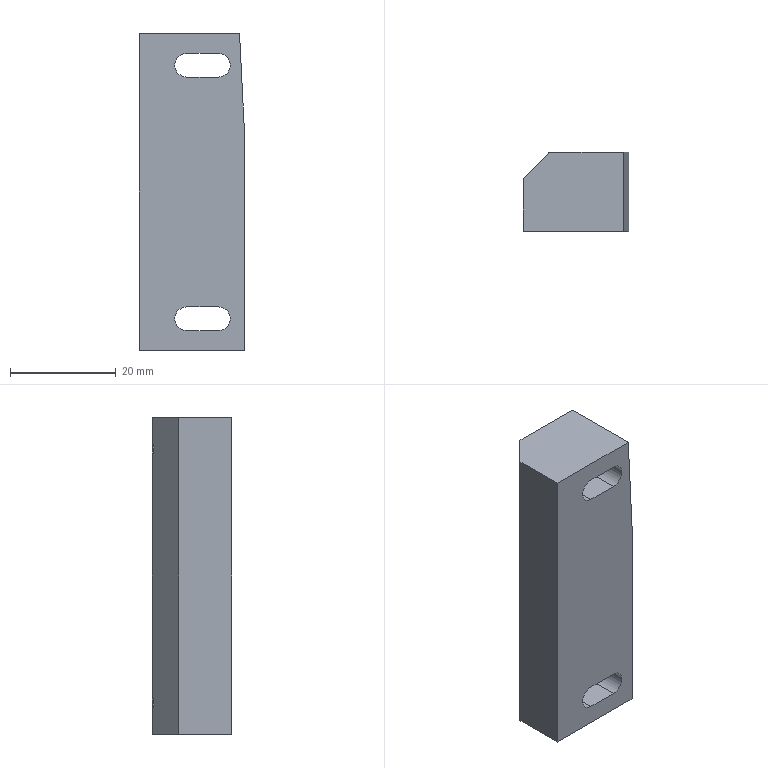Part | SolidWorks | features Cut 3, Chamfer 1, Extrusion 1, MirrorPattern 1 | 1 solid | 26 faces | box 20 x 15 x 60 mm | volume 15035 mm3 | plane 18 | cylinder 8 | commonest cylinder face diameters 4.5 x4 8.5 x4
STEP:
#1=CARTESIAN_POINT('',(-5.,15.,-22.564));
#2=VERTEX_POINT('',#1);
#3=CARTESIAN_POINT('',(-5.,15.,22.564));
#4=VERTEX_POINT('',#3);
#5=CARTESIAN_POINT('',(-5.,15.,30.));
#6=DIRECTION('',(0.,0.,1.));
#7=VECTOR('',#6,1000.);
#8=LINE('',#5,#7);
#9=EDGE_CURVE('',#2,#4,#8,.T.);
#10=ORIENTED_EDGE('',*,*,#9,.T.);
#11=CARTESIAN_POINT('',(-1.,15.,19.75));
#12=VERTEX_POINT('',#11);
#13=CARTESIAN_POINT('',(-1.,15.,24.));
#14=DIRECTION('',(0.,-1.,0.));
#15=DIRECTION('',(0.,0.,-1.));
#16=AXIS2_PLACEMENT_3D('',#13,#14,#15);
#17=CIRCLE('',#16,4.25);
#18=EDGE_CURVE('',#4,#12,#17,.T.);
#19=ORIENTED_EDGE('',*,*,#18,.T.);
#20=CARTESIAN_POINT('',(5.,15.,19.75));
#21=VERTEX_POINT('',#20);
#22=CARTESIAN_POINT('',(-1.,15.,19.75));
#23=DIRECTION('',(1.,0.,0.));
#24=VECTOR('',#23,1000.);
#25=LINE('',#22,#24);
#26=EDGE_CURVE('',#12,#21,#25,.T.);
#27=ORIENTED_EDGE('',*,*,#26,.T.);
#28=CARTESIAN_POINT('',(5.,15.,28.25));
#29=VERTEX_POINT('',#28);
#30=CARTESIAN_POINT('',(5.,15.,24.));
#31=DIRECTION('',(0.,-1.,0.));
#32=DIRECTION('',(0.,0.,-1.));
#33=AXIS2_PLACEMENT_3D('',#30,#31,#32);
#34=CIRCLE('',#33,4.25);
#35=EDGE_CURVE('',#21,#29,#34,.T.);
#36=ORIENTED_EDGE('',*,*,#35,.T.);
#37=CARTESIAN_POINT('',(-1.,15.,28.25));
#38=VERTEX_POINT('',#37);
#39=CARTESIAN_POINT('',(5.,15.,28.25));
#40=DIRECTION('',(-1.,0.,0.));
#41=VECTOR('',#40,1000.);
#42=LINE('',#39,#41);
#43=EDGE_CURVE('',#29,#38,#42,.T.);
#44=ORIENTED_EDGE('',*,*,#43,.T.);
#45=CARTESIAN_POINT('',(-5.,15.,25.436));
#46=VERTEX_POINT('',#45);
#47=CARTESIAN_POINT('',(-1.,15.,24.));
#48=DIRECTION('',(0.,-1.,0.));
#49=DIRECTION('',(0.,0.,-1.));
#50=AXIS2_PLACEMENT_3D('',#47,#48,#49);
#51=CIRCLE('',#50,4.25);
#52=EDGE_CURVE('',#38,#46,#51,.T.);
#53=ORIENTED_EDGE('',*,*,#52,.T.);
#54=CARTESIAN_POINT('',(-5.,15.,30.));
#55=VERTEX_POINT('',#54);
#56=CARTESIAN_POINT('',(-5.,15.,30.));
#57=DIRECTION('',(0.,0.,1.));
#58=VECTOR('',#57,1000.);
#59=LINE('',#56,#58);
#60=EDGE_CURVE('',#46,#55,#59,.T.);
#61=ORIENTED_EDGE('',*,*,#60,.T.);
#62=CARTESIAN_POINT('',(9.,15.,30.));
#63=VERTEX_POINT('',#62);
#64=CARTESIAN_POINT('',(-10.,15.,30.));
#65=DIRECTION('',(1.,0.,0.));
#66=VECTOR('',#65,1000.);
#67=LINE('',#64,#66);
#68=EDGE_CURVE('',#55,#63,#67,.T.);
#69=ORIENTED_EDGE('',*,*,#68,.T.);
#70=CARTESIAN_POINT('',(10.,15.,10.));
#71=VERTEX_POINT('',#70);
#72=CARTESIAN_POINT('',(9.,15.,30.));
#73=DIRECTION('',(-0.04994,0.,0.9988));
#74=VECTOR('',#73,1000.);
#75=LINE('',#72,#74);
#76=EDGE_CURVE('',#71,#63,#75,.T.);
#77=ORIENTED_EDGE('',*,*,#76,.F.);
#78=CARTESIAN_POINT('',(10.,15.,-30.));
#79=VERTEX_POINT('',#78);
#80=CARTESIAN_POINT('',(10.,15.,-30.));
#81=DIRECTION('',(0.,0.,-1.));
#82=VECTOR('',#81,1000.);
#83=LINE('',#80,#82);
#84=EDGE_CURVE('',#71,#79,#83,.T.);
#85=ORIENTED_EDGE('',*,*,#84,.T.);
#86=CARTESIAN_POINT('',(-5.,15.,-30.));
#87=VERTEX_POINT('',#86);
#88=CARTESIAN_POINT('',(-10.,15.,-30.));
#89=DIRECTION('',(-1.,0.,0.));
#90=VECTOR('',#89,1000.);
#91=LINE('',#88,#90);
#92=EDGE_CURVE('',#79,#87,#91,.T.);
#93=ORIENTED_EDGE('',*,*,#92,.T.);
#94=CARTESIAN_POINT('',(-5.,15.,-25.436));
#95=VERTEX_POINT('',#94);
#96=CARTESIAN_POINT('',(-5.,15.,30.));
#97=DIRECTION('',(0.,0.,1.));
#98=VECTOR('',#97,1000.);
#99=LINE('',#96,#98);
#100=EDGE_CURVE('',#87,#95,#99,.T.);
#101=ORIENTED_EDGE('',*,*,#100,.T.);
#102=CARTESIAN_POINT('',(-1.,15.,-28.25));
#103=VERTEX_POINT('',#102);
#104=CARTESIAN_POINT('',(-1.,15.,-24.));
#105=DIRECTION('',(0.,1.,0.));
#106=DIRECTION('',(0.,0.,1.));
#107=AXIS2_PLACEMENT_3D('',#104,#105,#106);
#108=CIRCLE('',#107,4.25);
#109=EDGE_CURVE('',#103,#95,#108,.T.);
#110=ORIENTED_EDGE('',*,*,#109,.F.);
#111=CARTESIAN_POINT('',(5.,15.,-28.25));
#112=VERTEX_POINT('',#111);
#113=CARTESIAN_POINT('',(5.,15.,-28.25));
#114=DIRECTION('',(-1.,0.,0.));
#115=VECTOR('',#114,1000.);
#116=LINE('',#113,#115);
#117=EDGE_CURVE('',#112,#103,#116,.T.);
#118=ORIENTED_EDGE('',*,*,#117,.F.);
#119=CARTESIAN_POINT('',(5.,15.,-19.75));
#120=VERTEX_POINT('',#119);
#121=CARTESIAN_POINT('',(5.,15.,-24.));
#122=DIRECTION('',(0.,1.,0.));
#123=DIRECTION('',(0.,0.,1.));
#124=AXIS2_PLACEMENT_3D('',#121,#122,#123);
#125=CIRCLE('',#124,4.25);
#126=EDGE_CURVE('',#120,#112,#125,.T.);
#127=ORIENTED_EDGE('',*,*,#126,.F.);
#128=CARTESIAN_POINT('',(-1.,15.,-19.75));
#129=VERTEX_POINT('',#128);
#130=CARTESIAN_POINT('',(-1.,15.,-19.75));
#131=DIRECTION('',(1.,0.,0.));
#132=VECTOR('',#131,1000.);
#133=LINE('',#130,#132);
#134=EDGE_CURVE('',#129,#120,#133,.T.);
#135=ORIENTED_EDGE('',*,*,#134,.F.);
#136=CARTESIAN_POINT('',(-1.,15.,-24.));
#137=DIRECTION('',(0.,1.,0.));
#138=DIRECTION('',(0.,0.,1.));
#139=AXIS2_PLACEMENT_3D('',#136,#137,#138);
#140=CIRCLE('',#139,4.25);
#141=EDGE_CURVE('',#2,#129,#140,.T.);
#142=ORIENTED_EDGE('',*,*,#141,.F.);
#143=EDGE_LOOP('',(#10,#19,#27,#36,#44,#53,#61,#69,#77,#85,#93,#101,#110,#118,#127,#135,#142));
#144=FACE_OUTER_BOUND('',#143,.T.);
#145=CARTESIAN_POINT('',(0.,15.,0.));
#146=DIRECTION('',(0.,1.,0.));
#147=DIRECTION('',(0.,0.,1.));
#148=AXIS2_PLACEMENT_3D('',#145,#146,#147);
#149=PLANE('',#148);
#150=ADVANCED_FACE('',(#144),#149,.T.);
#151=ORIENTED_EDGE('',*,*,#60,.F.);
#152=CARTESIAN_POINT('',(-5.,15.,25.436));
#153=CARTESIAN_POINT('',(-5.337,14.663,24.498));
#154=CARTESIAN_POINT('',(-5.337,14.663,23.502));
#155=CARTESIAN_POINT('',(-5.,15.,22.564));
#156=(BOUNDED_CURVE()B_SPLINE_CURVE(3,(#152,#153,#154,#155),.UNSPECIFIED.,.F.,.F.)B_SPLINE_CURVE_WITH_KNOTS((4,4),(2.797,3.486),.UNSPECIFIED.)CURVE()GEOMETRIC_REPRESENTATION_ITEM()RATIONAL_B_SPLINE_CURVE((1.,0.9608,0.9608,1.))REPRESENTATION_ITEM(''));
#157=EDGE_CURVE('',#46,#4,#156,.T.);
#158=ORIENTED_EDGE('',*,*,#157,.T.);
#159=ORIENTED_EDGE('',*,*,#9,.F.);
#160=CARTESIAN_POINT('',(-5.,15.,-25.436));
#161=CARTESIAN_POINT('',(-5.337,14.663,-24.498));
#162=CARTESIAN_POINT('',(-5.337,14.663,-23.502));
#163=CARTESIAN_POINT('',(-5.,15.,-22.564));
#164=(BOUNDED_CURVE()B_SPLINE_CURVE(3,(#160,#161,#162,#163),.UNSPECIFIED.,.F.,.F.)B_SPLINE_CURVE_WITH_KNOTS((4,4),(2.797,3.486),.UNSPECIFIED.)CURVE()GEOMETRIC_REPRESENTATION_ITEM()RATIONAL_B_SPLINE_CURVE((1.,0.9608,0.9608,1.))REPRESENTATION_ITEM(''));
#165=EDGE_CURVE('',#95,#2,#164,.T.);
#166=ORIENTED_EDGE('',*,*,#165,.F.);
#167=ORIENTED_EDGE('',*,*,#100,.F.);
#168=CARTESIAN_POINT('',(-10.,10.,-30.));
#169=VERTEX_POINT('',#168);
#170=CARTESIAN_POINT('',(-5.,15.,-30.));
#171=DIRECTION('',(0.7071,0.7071,0.));
#172=VECTOR('',#171,1000.);
#173=LINE('',#170,#172);
#174=EDGE_CURVE('',#169,#87,#173,.T.);
#175=ORIENTED_EDGE('',*,*,#174,.F.);
#176=CARTESIAN_POINT('',(-10.,10.,30.));
#177=VERTEX_POINT('',#176);
#178=CARTESIAN_POINT('',(-10.,10.,-30.));
#179=DIRECTION('',(0.,0.,-1.));
#180=VECTOR('',#179,1000.);
#181=LINE('',#178,#180);
#182=EDGE_CURVE('',#177,#169,#181,.T.);
#183=ORIENTED_EDGE('',*,*,#182,.F.);
#184=CARTESIAN_POINT('',(-5.,15.,30.));
#185=DIRECTION('',(-0.7071,-0.7071,0.));
#186=VECTOR('',#185,1000.);
#187=LINE('',#184,#186);
#188=EDGE_CURVE('',#55,#177,#187,.T.);
#189=ORIENTED_EDGE('',*,*,#188,.F.);
#190=EDGE_LOOP('',(#151,#158,#159,#166,#167,#175,#183,#189));
#191=FACE_OUTER_BOUND('',#190,.T.);
#192=CARTESIAN_POINT('',(-5.,15.,0.));
#193=DIRECTION('',(-0.7071,0.7071,0.));
#194=DIRECTION('',(0.,0.,-1.));
#195=AXIS2_PLACEMENT_3D('',#192,#193,#194);
#196=PLANE('',#195);
#197=ADVANCED_FACE('',(#191),#196,.T.);
#198=CARTESIAN_POINT('',(5.,0.,26.25));
#199=VERTEX_POINT('',#198);
#200=CARTESIAN_POINT('',(5.,9.,26.25));
#201=VERTEX_POINT('',#200);
#202=CARTESIAN_POINT('',(5.,0.,26.25));
#203=DIRECTION('',(0.,1.,0.));
#204=VECTOR('',#203,1000.);
#205=LINE('',#202,#204);
#206=EDGE_CURVE('',#199,#201,#205,.T.);
#207=ORIENTED_EDGE('',*,*,#206,.T.);
#208=CARTESIAN_POINT('',(5.,9.,21.75));
#209=VERTEX_POINT('',#208);
#210=CARTESIAN_POINT('',(5.,9.,24.));
#211=DIRECTION('',(0.,1.,0.));
#212=DIRECTION('',(0.,0.,1.));
#213=AXIS2_PLACEMENT_3D('',#210,#211,#212);
#214=CIRCLE('',#213,2.25);
#215=EDGE_CURVE('',#201,#209,#214,.T.);
#216=ORIENTED_EDGE('',*,*,#215,.T.);
#217=CARTESIAN_POINT('',(5.,0.,21.75));
#218=VERTEX_POINT('',#217);
#219=CARTESIAN_POINT('',(5.,0.,21.75));
#220=DIRECTION('',(0.,1.,0.));
#221=VECTOR('',#220,1000.);
#222=LINE('',#219,#221);
#223=EDGE_CURVE('',#218,#209,#222,.T.);
#224=ORIENTED_EDGE('',*,*,#223,.F.);
#225=CARTESIAN_POINT('',(5.,0.,24.));
#226=DIRECTION('',(0.,-1.,0.));
#227=DIRECTION('',(0.,0.,-1.));
#228=AXIS2_PLACEMENT_3D('',#225,#226,#227);
#229=CIRCLE('',#228,2.25);
#230=EDGE_CURVE('',#218,#199,#229,.T.);
#231=ORIENTED_EDGE('',*,*,#230,.T.);
#232=EDGE_LOOP('',(#207,#216,#224,#231));
#233=FACE_OUTER_BOUND('',#232,.T.);
#234=CARTESIAN_POINT('',(5.,0.,24.));
#235=DIRECTION('',(0.,1.,0.));
#236=DIRECTION('',(0.,0.,1.));
#237=AXIS2_PLACEMENT_3D('',#234,#235,#236);
#238=CYLINDRICAL_SURFACE('',#237,2.25);
#239=ADVANCED_FACE('',(#233),#238,.F.);
#240=CARTESIAN_POINT('',(-1.,0.,26.25));
#241=VERTEX_POINT('',#240);
#242=CARTESIAN_POINT('',(-1.,9.,26.25));
#243=VERTEX_POINT('',#242);
#244=CARTESIAN_POINT('',(-1.,0.,26.25));
#245=DIRECTION('',(0.,1.,0.));
#246=VECTOR('',#245,1000.);
#247=LINE('',#244,#246);
#248=EDGE_CURVE('',#241,#243,#247,.T.);
#249=ORIENTED_EDGE('',*,*,#248,.T.);
#250=CARTESIAN_POINT('',(5.,9.,26.25));
#251=DIRECTION('',(1.,0.,0.));
#252=VECTOR('',#251,1000.);
#253=LINE('',#250,#252);
#254=EDGE_CURVE('',#243,#201,#253,.T.);
#255=ORIENTED_EDGE('',*,*,#254,.T.);
#256=ORIENTED_EDGE('',*,*,#206,.F.);
#257=CARTESIAN_POINT('',(5.,0.,26.25));
#258=DIRECTION('',(-1.,0.,0.));
#259=VECTOR('',#258,1000.);
#260=LINE('',#257,#259);
#261=EDGE_CURVE('',#199,#241,#260,.T.);
#262=ORIENTED_EDGE('',*,*,#261,.T.);
#263=EDGE_LOOP('',(#249,#255,#256,#262));
#264=FACE_OUTER_BOUND('',#263,.T.);
#265=CARTESIAN_POINT('',(5.,0.,26.25));
#266=DIRECTION('',(0.,0.,-1.));
#267=DIRECTION('',(-1.,0.,0.));
#268=AXIS2_PLACEMENT_3D('',#265,#266,#267);
#269=PLANE('',#268);
#270=ADVANCED_FACE('',(#264),#269,.T.);
#271=CARTESIAN_POINT('',(-1.,0.,21.75));
#272=VERTEX_POINT('',#271);
#273=CARTESIAN_POINT('',(-1.,9.,21.75));
#274=VERTEX_POINT('',#273);
#275=CARTESIAN_POINT('',(-1.,0.,21.75));
#276=DIRECTION('',(0.,1.,0.));
#277=VECTOR('',#276,1000.);
#278=LINE('',#275,#277);
#279=EDGE_CURVE('',#272,#274,#278,.T.);
#280=ORIENTED_EDGE('',*,*,#279,.T.);
#281=CARTESIAN_POINT('',(-1.,9.,24.));
#282=DIRECTION('',(0.,1.,0.));
#283=DIRECTION('',(0.,0.,1.));
#284=AXIS2_PLACEMENT_3D('',#281,#282,#283);
#285=CIRCLE('',#284,2.25);
#286=EDGE_CURVE('',#274,#243,#285,.T.);
#287=ORIENTED_EDGE('',*,*,#286,.T.);
#288=ORIENTED_EDGE('',*,*,#248,.F.);
#289=CARTESIAN_POINT('',(-1.,0.,24.));
#290=DIRECTION('',(0.,-1.,0.));
#291=DIRECTION('',(0.,0.,-1.));
#292=AXIS2_PLACEMENT_3D('',#289,#290,#291);
#293=CIRCLE('',#292,2.25);
#294=EDGE_CURVE('',#241,#272,#293,.T.);
#295=ORIENTED_EDGE('',*,*,#294,.T.);
#296=EDGE_LOOP('',(#280,#287,#288,#295));
#297=FACE_OUTER_BOUND('',#296,.T.);
#298=CARTESIAN_POINT('',(-1.,0.,24.));
#299=DIRECTION('',(0.,1.,0.));
#300=DIRECTION('',(0.,0.,1.));
#301=AXIS2_PLACEMENT_3D('',#298,#299,#300);
#302=CYLINDRICAL_SURFACE('',#301,2.25);
#303=ADVANCED_FACE('',(#297),#302,.F.);
#304=ORIENTED_EDGE('',*,*,#223,.T.);
#305=CARTESIAN_POINT('',(5.,9.,21.75));
#306=DIRECTION('',(-1.,0.,0.));
#307=VECTOR('',#306,1000.);
#308=LINE('',#305,#307);
#309=EDGE_CURVE('',#209,#274,#308,.T.);
#310=ORIENTED_EDGE('',*,*,#309,.T.);
#311=ORIENTED_EDGE('',*,*,#279,.F.);
#312=CARTESIAN_POINT('',(5.,0.,21.75));
#313=DIRECTION('',(1.,0.,0.));
#314=VECTOR('',#313,1000.);
#315=LINE('',#312,#314);
#316=EDGE_CURVE('',#272,#218,#315,.T.);
#317=ORIENTED_EDGE('',*,*,#316,.T.);
#318=EDGE_LOOP('',(#304,#310,#311,#317));
#319=FACE_OUTER_BOUND('',#318,.T.);
#320=CARTESIAN_POINT('',(5.,0.,21.75));
#321=DIRECTION('',(0.,0.,1.));
#322=DIRECTION('',(1.,0.,0.));
#323=AXIS2_PLACEMENT_3D('',#320,#321,#322);
#324=PLANE('',#323);
#325=ADVANCED_FACE('',(#319),#324,.T.);
#326=CARTESIAN_POINT('',(10.,0.,10.));
#327=VERTEX_POINT('',#326);
#328=CARTESIAN_POINT('',(10.,0.,-30.));
#329=VERTEX_POINT('',#328);
#330=CARTESIAN_POINT('',(10.,0.,-30.));
#331=DIRECTION('',(0.,0.,-1.));
#332=VECTOR('',#331,1000.);
#333=LINE('',#330,#332);
#334=EDGE_CURVE('',#327,#329,#333,.T.);
#335=ORIENTED_EDGE('',*,*,#334,.F.);
#336=CARTESIAN_POINT('',(9.,0.,30.));
#337=VERTEX_POINT('',#336);
#338=CARTESIAN_POINT('',(9.,0.,30.));
#339=DIRECTION('',(-0.04994,0.,0.9988));
#340=VECTOR('',#339,1000.);
#341=LINE('',#338,#340);
#342=EDGE_CURVE('',#327,#337,#341,.T.);
#343=ORIENTED_EDGE('',*,*,#342,.T.);
#344=CARTESIAN_POINT('',(-10.,0.,30.));
#345=VERTEX_POINT('',#344);
#346=CARTESIAN_POINT('',(-10.,0.,30.));
#347=DIRECTION('',(1.,0.,0.));
#348=VECTOR('',#347,1000.);
#349=LINE('',#346,#348);
#350=EDGE_CURVE('',#345,#337,#349,.T.);
#351=ORIENTED_EDGE('',*,*,#350,.F.);
#352=CARTESIAN_POINT('',(-10.,0.,-30.));
#353=VERTEX_POINT('',#352);
#354=CARTESIAN_POINT('',(-10.,0.,-30.));
#355=DIRECTION('',(0.,0.,1.));
#356=VECTOR('',#355,1000.);
#357=LINE('',#354,#356);
#358=EDGE_CURVE('',#353,#345,#357,.T.);
#359=ORIENTED_EDGE('',*,*,#358,.F.);
#360=CARTESIAN_POINT('',(-10.,0.,-30.));
#361=DIRECTION('',(-1.,0.,0.));
#362=VECTOR('',#361,1000.);
#363=LINE('',#360,#362);
#364=EDGE_CURVE('',#329,#353,#363,.T.);
#365=ORIENTED_EDGE('',*,*,#364,.F.);
#366=EDGE_LOOP('',(#335,#343,#351,#359,#365));
#367=FACE_OUTER_BOUND('',#366,.T.);
#368=CARTESIAN_POINT('',(-1.,0.,-21.75));
#369=VERTEX_POINT('',#368);
#370=CARTESIAN_POINT('',(5.,0.,-21.75));
#371=VERTEX_POINT('',#370);
#372=CARTESIAN_POINT('',(5.,0.,-21.75));
#373=DIRECTION('',(1.,0.,0.));
#374=VECTOR('',#373,1000.);
#375=LINE('',#372,#374);
#376=EDGE_CURVE('',#369,#371,#375,.T.);
#377=ORIENTED_EDGE('',*,*,#376,.T.);
#378=CARTESIAN_POINT('',(5.,0.,-26.25));
#379=VERTEX_POINT('',#378);
#380=CARTESIAN_POINT('',(5.,0.,-24.));
#381=DIRECTION('',(0.,1.,0.));
#382=DIRECTION('',(0.,0.,1.));
#383=AXIS2_PLACEMENT_3D('',#380,#381,#382);
#384=CIRCLE('',#383,2.25);
#385=EDGE_CURVE('',#371,#379,#384,.T.);
#386=ORIENTED_EDGE('',*,*,#385,.T.);
#387=CARTESIAN_POINT('',(-1.,0.,-26.25));
#388=VERTEX_POINT('',#387);
#389=CARTESIAN_POINT('',(5.,0.,-26.25));
#390=DIRECTION('',(-1.,0.,0.));
#391=VECTOR('',#390,1000.);
#392=LINE('',#389,#391);
#393=EDGE_CURVE('',#379,#388,#392,.T.);
#394=ORIENTED_EDGE('',*,*,#393,.T.);
#395=CARTESIAN_POINT('',(-1.,0.,-24.));
#396=DIRECTION('',(0.,1.,0.));
#397=DIRECTION('',(0.,0.,1.));
#398=AXIS2_PLACEMENT_3D('',#395,#396,#397);
#399=CIRCLE('',#398,2.25);
#400=EDGE_CURVE('',#388,#369,#399,.T.);
#401=ORIENTED_EDGE('',*,*,#400,.T.);
#402=EDGE_LOOP('',(#377,#386,#394,#401));
#403=FACE_BOUND('',#402,.T.);
#404=ORIENTED_EDGE('',*,*,#230,.F.);
#405=ORIENTED_EDGE('',*,*,#316,.F.);
#406=ORIENTED_EDGE('',*,*,#294,.F.);
#407=ORIENTED_EDGE('',*,*,#261,.F.);
#408=EDGE_LOOP('',(#404,#405,#406,#407));
#409=FACE_BOUND('',#408,.T.);
#410=CARTESIAN_POINT('',(0.,0.,0.));
#411=DIRECTION('',(0.,1.,0.));
#412=DIRECTION('',(0.,0.,1.));
#413=AXIS2_PLACEMENT_3D('',#410,#411,#412);
#414=PLANE('',#413);
#415=ADVANCED_FACE('',(#367,#403,#409),#414,.F.);
#416=CARTESIAN_POINT('',(5.,9.,-26.25));
#417=VERTEX_POINT('',#416);
#418=CARTESIAN_POINT('',(5.,9.,-21.75));
#419=VERTEX_POINT('',#418);
#420=CARTESIAN_POINT('',(5.,9.,-24.));
#421=DIRECTION('',(0.,-1.,0.));
#422=DIRECTION('',(0.,0.,1.));
#423=AXIS2_PLACEMENT_3D('',#420,#421,#422);
#424=CIRCLE('',#423,2.25);
#425=EDGE_CURVE('',#417,#419,#424,.T.);
#426=ORIENTED_EDGE('',*,*,#425,.F.);
#427=CARTESIAN_POINT('',(5.,0.,-26.25));
#428=DIRECTION('',(0.,1.,0.));
#429=VECTOR('',#428,1000.);
#430=LINE('',#427,#429);
#431=EDGE_CURVE('',#379,#417,#430,.T.);
#432=ORIENTED_EDGE('',*,*,#431,.F.);
#433=ORIENTED_EDGE('',*,*,#385,.F.);
#434=CARTESIAN_POINT('',(5.,0.,-21.75));
#435=DIRECTION('',(0.,1.,0.));
#436=VECTOR('',#435,1000.);
#437=LINE('',#434,#436);
#438=EDGE_CURVE('',#371,#419,#437,.T.);
#439=ORIENTED_EDGE('',*,*,#438,.T.);
#440=EDGE_LOOP('',(#426,#432,#433,#439));
#441=FACE_OUTER_BOUND('',#440,.T.);
#442=CARTESIAN_POINT('',(5.,0.,-24.));
#443=DIRECTION('',(0.,1.,0.));
#444=DIRECTION('',(0.,0.,1.));
#445=AXIS2_PLACEMENT_3D('',#442,#443,#444);
#446=CYLINDRICAL_SURFACE('',#445,2.25);
#447=ADVANCED_FACE('',(#441),#446,.F.);
#448=CARTESIAN_POINT('',(-1.,9.,-21.75));
#449=VERTEX_POINT('',#448);
#450=CARTESIAN_POINT('',(5.,9.,-21.75));
#451=DIRECTION('',(-1.,0.,0.));
#452=VECTOR('',#451,1000.);
#453=LINE('',#450,#452);
#454=EDGE_CURVE('',#419,#449,#453,.T.);
#455=ORIENTED_EDGE('',*,*,#454,.F.);
#456=ORIENTED_EDGE('',*,*,#438,.F.);
#457=ORIENTED_EDGE('',*,*,#376,.F.);
#458=CARTESIAN_POINT('',(-1.,0.,-21.75));
#459=DIRECTION('',(0.,1.,0.));
#460=VECTOR('',#459,1000.);
#461=LINE('',#458,#460);
#462=EDGE_CURVE('',#369,#449,#461,.T.);
#463=ORIENTED_EDGE('',*,*,#462,.T.);
#464=EDGE_LOOP('',(#455,#456,#457,#463));
#465=FACE_OUTER_BOUND('',#464,.T.);
#466=CARTESIAN_POINT('',(5.,0.,-21.75));
#467=DIRECTION('',(0.,0.,1.));
#468=DIRECTION('',(1.,0.,0.));
#469=AXIS2_PLACEMENT_3D('',#466,#467,#468);
#470=PLANE('',#469);
#471=ADVANCED_FACE('',(#465),#470,.F.);
#472=CARTESIAN_POINT('',(-1.,9.,-26.25));
#473=VERTEX_POINT('',#472);
#474=CARTESIAN_POINT('',(-1.,9.,-24.));
#475=DIRECTION('',(0.,-1.,0.));
#476=DIRECTION('',(0.,0.,1.));
#477=AXIS2_PLACEMENT_3D('',#474,#475,#476);
#478=CIRCLE('',#477,2.25);
#479=EDGE_CURVE('',#449,#473,#478,.T.);
#480=ORIENTED_EDGE('',*,*,#479,.F.);
#481=ORIENTED_EDGE('',*,*,#462,.F.);
#482=ORIENTED_EDGE('',*,*,#400,.F.);
#483=CARTESIAN_POINT('',(-1.,0.,-26.25));
#484=DIRECTION('',(0.,1.,0.));
#485=VECTOR('',#484,1000.);
#486=LINE('',#483,#485);
#487=EDGE_CURVE('',#388,#473,#486,.T.);
#488=ORIENTED_EDGE('',*,*,#487,.T.);
#489=EDGE_LOOP('',(#480,#481,#482,#488));
#490=FACE_OUTER_BOUND('',#489,.T.);
#491=CARTESIAN_POINT('',(-1.,0.,-24.));
#492=DIRECTION('',(0.,1.,0.));
#493=DIRECTION('',(0.,0.,1.));
#494=AXIS2_PLACEMENT_3D('',#491,#492,#493);
#495=CYLINDRICAL_SURFACE('',#494,2.25);
#496=ADVANCED_FACE('',(#490),#495,.F.);
#497=CARTESIAN_POINT('',(5.,9.,-26.25));
#498=DIRECTION('',(1.,0.,0.));
#499=VECTOR('',#498,1000.);
#500=LINE('',#497,#499);
#501=EDGE_CURVE('',#473,#417,#500,.T.);
#502=ORIENTED_EDGE('',*,*,#501,.F.);
#503=ORIENTED_EDGE('',*,*,#487,.F.);
#504=ORIENTED_EDGE('',*,*,#393,.F.);
#505=ORIENTED_EDGE('',*,*,#431,.T.);
#506=EDGE_LOOP('',(#502,#503,#504,#505));
#507=FACE_OUTER_BOUND('',#506,.T.);
#508=CARTESIAN_POINT('',(5.,0.,-26.25));
#509=DIRECTION('',(0.,0.,-1.));
#510=DIRECTION('',(-1.,0.,0.));
#511=AXIS2_PLACEMENT_3D('',#508,#509,#510);
#512=PLANE('',#511);
#513=ADVANCED_FACE('',(#507),#512,.F.);
#514=ORIENTED_EDGE('',*,*,#84,.F.);
#515=CARTESIAN_POINT('',(10.,0.,10.));
#516=DIRECTION('',(0.,1.,0.));
#517=VECTOR('',#516,1000.);
#518=LINE('',#515,#517);
#519=EDGE_CURVE('',#327,#71,#518,.T.);
#520=ORIENTED_EDGE('',*,*,#519,.F.);
#521=ORIENTED_EDGE('',*,*,#334,.T.);
#522=CARTESIAN_POINT('',(10.,15.,-30.));
#523=DIRECTION('',(0.,-1.,0.));
#524=VECTOR('',#523,1000.);
#525=LINE('',#522,#524);
#526=EDGE_CURVE('',#79,#329,#525,.T.);
#527=ORIENTED_EDGE('',*,*,#526,.F.);
#528=EDGE_LOOP('',(#514,#520,#521,#527));
#529=FACE_OUTER_BOUND('',#528,.T.);
#530=CARTESIAN_POINT('',(10.,15.,-30.));
#531=DIRECTION('',(-1.,0.,0.));
#532=DIRECTION('',(0.,0.,1.));
#533=AXIS2_PLACEMENT_3D('',#530,#531,#532);
#534=PLANE('',#533);
#535=ADVANCED_FACE('',(#529),#534,.F.);
#536=CARTESIAN_POINT('',(-10.,15.,-30.));
#537=DIRECTION('',(0.,-1.,0.));
#538=VECTOR('',#537,1000.);
#539=LINE('',#536,#538);
#540=EDGE_CURVE('',#169,#353,#539,.T.);
#541=ORIENTED_EDGE('',*,*,#540,.F.);
#542=ORIENTED_EDGE('',*,*,#174,.T.);
#543=ORIENTED_EDGE('',*,*,#92,.F.);
#544=ORIENTED_EDGE('',*,*,#526,.T.);
#545=ORIENTED_EDGE('',*,*,#364,.T.);
#546=EDGE_LOOP('',(#541,#542,#543,#544,#545));
#547=FACE_OUTER_BOUND('',#546,.T.);
#548=CARTESIAN_POINT('',(-10.,15.,-30.));
#549=DIRECTION('',(0.,0.,1.));
#550=DIRECTION('',(1.,0.,0.));
#551=AXIS2_PLACEMENT_3D('',#548,#549,#550);
#552=PLANE('',#551);
#553=ADVANCED_FACE('',(#547),#552,.F.);
#554=CARTESIAN_POINT('',(-10.,15.,30.));
#555=DIRECTION('',(0.,-1.,0.));
#556=VECTOR('',#555,1000.);
#557=LINE('',#554,#556);
#558=EDGE_CURVE('',#177,#345,#557,.T.);
#559=ORIENTED_EDGE('',*,*,#558,.F.);
#560=ORIENTED_EDGE('',*,*,#182,.T.);
#561=ORIENTED_EDGE('',*,*,#540,.T.);
#562=ORIENTED_EDGE('',*,*,#358,.T.);
#563=EDGE_LOOP('',(#559,#560,#561,#562));
#564=FACE_OUTER_BOUND('',#563,.T.);
#565=CARTESIAN_POINT('',(-10.,15.,-30.));
#566=DIRECTION('',(1.,0.,0.));
#567=DIRECTION('',(0.,0.,-1.));
#568=AXIS2_PLACEMENT_3D('',#565,#566,#567);
#569=PLANE('',#568);
#570=ADVANCED_FACE('',(#564),#569,.F.);
#571=ORIENTED_EDGE('',*,*,#350,.T.);
#572=CARTESIAN_POINT('',(9.,0.,30.));
#573=DIRECTION('',(0.,1.,0.));
#574=VECTOR('',#573,1000.);
#575=LINE('',#572,#574);
#576=EDGE_CURVE('',#337,#63,#575,.T.);
#577=ORIENTED_EDGE('',*,*,#576,.T.);
#578=ORIENTED_EDGE('',*,*,#68,.F.);
#579=ORIENTED_EDGE('',*,*,#188,.T.);
#580=ORIENTED_EDGE('',*,*,#558,.T.);
#581=EDGE_LOOP('',(#571,#577,#578,#579,#580));
#582=FACE_OUTER_BOUND('',#581,.T.);
#583=CARTESIAN_POINT('',(-10.,15.,30.));
#584=DIRECTION('',(0.,0.,-1.));
#585=DIRECTION('',(-1.,0.,0.));
#586=AXIS2_PLACEMENT_3D('',#583,#584,#585);
#587=PLANE('',#586);
#588=ADVANCED_FACE('',(#582),#587,.F.);
#589=ORIENTED_EDGE('',*,*,#76,.T.);
#590=ORIENTED_EDGE('',*,*,#576,.F.);
#591=ORIENTED_EDGE('',*,*,#342,.F.);
#592=ORIENTED_EDGE('',*,*,#519,.T.);
#593=EDGE_LOOP('',(#589,#590,#591,#592));
#594=FACE_OUTER_BOUND('',#593,.T.);
#595=CARTESIAN_POINT('',(9.,0.,30.));
#596=DIRECTION('',(-0.9988,0.,-0.04994));
#597=DIRECTION('',(-0.04994,0.,0.9988));
#598=AXIS2_PLACEMENT_3D('',#595,#596,#597);
#599=PLANE('',#598);
#600=ADVANCED_FACE('',(#594),#599,.F.);
#601=CARTESIAN_POINT('',(-1.,9.,-28.25));
#602=VERTEX_POINT('',#601);
#603=CARTESIAN_POINT('',(-1.,9.,-19.75));
#604=VERTEX_POINT('',#603);
#605=CARTESIAN_POINT('',(-1.,9.,-24.));
#606=DIRECTION('',(0.,1.,0.));
#607=DIRECTION('',(0.,0.,1.));
#608=AXIS2_PLACEMENT_3D('',#605,#606,#607);
#609=CIRCLE('',#608,4.25);
#610=EDGE_CURVE('',#602,#604,#609,.T.);
#611=ORIENTED_EDGE('',*,*,#610,.T.);
#612=CARTESIAN_POINT('',(5.,9.,-19.75));
#613=VERTEX_POINT('',#612);
#614=CARTESIAN_POINT('',(-1.,9.,-19.75));
#615=DIRECTION('',(1.,0.,0.));
#616=VECTOR('',#615,1000.);
#617=LINE('',#614,#616);
#618=EDGE_CURVE('',#604,#613,#617,.T.);
#619=ORIENTED_EDGE('',*,*,#618,.T.);
#620=CARTESIAN_POINT('',(5.,9.,-28.25));
#621=VERTEX_POINT('',#620);
#622=CARTESIAN_POINT('',(5.,9.,-24.));
#623=DIRECTION('',(0.,1.,0.));
#624=DIRECTION('',(0.,0.,1.));
#625=AXIS2_PLACEMENT_3D('',#622,#623,#624);
#626=CIRCLE('',#625,4.25);
#627=EDGE_CURVE('',#613,#621,#626,.T.);
#628=ORIENTED_EDGE('',*,*,#627,.T.);
#629=CARTESIAN_POINT('',(5.,9.,-28.25));
#630=DIRECTION('',(-1.,0.,0.));
#631=VECTOR('',#630,1000.);
#632=LINE('',#629,#631);
#633=EDGE_CURVE('',#621,#602,#632,.T.);
#634=ORIENTED_EDGE('',*,*,#633,.T.);
#635=EDGE_LOOP('',(#611,#619,#628,#634));
#636=FACE_OUTER_BOUND('',#635,.T.);
#637=ORIENTED_EDGE('',*,*,#425,.T.);
#638=ORIENTED_EDGE('',*,*,#454,.T.);
#639=ORIENTED_EDGE('',*,*,#479,.T.);
#640=ORIENTED_EDGE('',*,*,#501,.T.);
#641=EDGE_LOOP('',(#637,#638,#639,#640));
#642=FACE_BOUND('',#641,.T.);
#643=CARTESIAN_POINT('',(-1.,9.,-24.));
#644=DIRECTION('',(0.,1.,0.));
#645=DIRECTION('',(0.,0.,1.));
#646=AXIS2_PLACEMENT_3D('',#643,#644,#645);
#647=PLANE('',#646);
#648=ADVANCED_FACE('',(#636,#642),#647,.T.);
#649=ORIENTED_EDGE('',*,*,#165,.T.);
#650=ORIENTED_EDGE('',*,*,#141,.T.);
#651=CARTESIAN_POINT('',(-1.,9.,-19.75));
#652=DIRECTION('',(0.,1.,0.));
#653=VECTOR('',#652,1000.);
#654=LINE('',#651,#653);
#655=EDGE_CURVE('',#604,#129,#654,.T.);
#656=ORIENTED_EDGE('',*,*,#655,.F.);
#657=ORIENTED_EDGE('',*,*,#610,.F.);
#658=CARTESIAN_POINT('',(-1.,9.,-28.25));
#659=DIRECTION('',(0.,1.,0.));
#660=VECTOR('',#659,1000.);
#661=LINE('',#658,#660);
#662=EDGE_CURVE('',#602,#103,#661,.T.);
#663=ORIENTED_EDGE('',*,*,#662,.T.);
#664=ORIENTED_EDGE('',*,*,#109,.T.);
#665=EDGE_LOOP('',(#649,#650,#656,#657,#663,#664));
#666=FACE_OUTER_BOUND('',#665,.T.);
#667=CARTESIAN_POINT('',(-1.,9.,-24.));
#668=DIRECTION('',(0.,1.,0.));
#669=DIRECTION('',(0.,0.,1.));
#670=AXIS2_PLACEMENT_3D('',#667,#668,#669);
#671=CYLINDRICAL_SURFACE('',#670,4.25);
#672=ADVANCED_FACE('',(#666),#671,.F.);
#673=ORIENTED_EDGE('',*,*,#117,.T.);
#674=ORIENTED_EDGE('',*,*,#662,.F.);
#675=ORIENTED_EDGE('',*,*,#633,.F.);
#676=CARTESIAN_POINT('',(5.,9.,-28.25));
#677=DIRECTION('',(0.,1.,0.));
#678=VECTOR('',#677,1000.);
#679=LINE('',#676,#678);
#680=EDGE_CURVE('',#621,#112,#679,.T.);
#681=ORIENTED_EDGE('',*,*,#680,.T.);
#682=EDGE_LOOP('',(#673,#674,#675,#681));
#683=FACE_OUTER_BOUND('',#682,.T.);
#684=CARTESIAN_POINT('',(5.,9.,-28.25));
#685=DIRECTION('',(0.,0.,-1.));
#686=DIRECTION('',(-1.,0.,0.));
#687=AXIS2_PLACEMENT_3D('',#684,#685,#686);
#688=PLANE('',#687);
#689=ADVANCED_FACE('',(#683),#688,.F.);
#690=ORIENTED_EDGE('',*,*,#126,.T.);
#691=ORIENTED_EDGE('',*,*,#680,.F.);
#692=ORIENTED_EDGE('',*,*,#627,.F.);
#693=CARTESIAN_POINT('',(5.,9.,-19.75));
#694=DIRECTION('',(0.,1.,0.));
#695=VECTOR('',#694,1000.);
#696=LINE('',#693,#695);
#697=EDGE_CURVE('',#613,#120,#696,.T.);
#698=ORIENTED_EDGE('',*,*,#697,.T.);
#699=EDGE_LOOP('',(#690,#691,#692,#698));
#700=FACE_OUTER_BOUND('',#699,.T.);
#701=CARTESIAN_POINT('',(5.,9.,-24.));
#702=DIRECTION('',(0.,1.,0.));
#703=DIRECTION('',(0.,0.,1.));
#704=AXIS2_PLACEMENT_3D('',#701,#702,#703);
#705=CYLINDRICAL_SURFACE('',#704,4.25);
#706=ADVANCED_FACE('',(#700),#705,.F.);
#707=ORIENTED_EDGE('',*,*,#134,.T.);
#708=ORIENTED_EDGE('',*,*,#697,.F.);
#709=ORIENTED_EDGE('',*,*,#618,.F.);
#710=ORIENTED_EDGE('',*,*,#655,.T.);
#711=EDGE_LOOP('',(#707,#708,#709,#710));
#712=FACE_OUTER_BOUND('',#711,.T.);
#713=CARTESIAN_POINT('',(-1.,9.,-19.75));
#714=DIRECTION('',(0.,0.,1.));
#715=DIRECTION('',(1.,0.,0.));
#716=AXIS2_PLACEMENT_3D('',#713,#714,#715);
#717=PLANE('',#716);
#718=ADVANCED_FACE('',(#712),#717,.F.);
#719=ORIENTED_EDGE('',*,*,#52,.F.);
#720=CARTESIAN_POINT('',(-1.,9.,28.25));
#721=VERTEX_POINT('',#720);
#722=CARTESIAN_POINT('',(-1.,9.,28.25));
#723=DIRECTION('',(0.,1.,0.));
#724=VECTOR('',#723,1000.);
#725=LINE('',#722,#724);
#726=EDGE_CURVE('',#721,#38,#725,.T.);
#727=ORIENTED_EDGE('',*,*,#726,.F.);
#728=CARTESIAN_POINT('',(-1.,9.,19.75));
#729=VERTEX_POINT('',#728);
#730=CARTESIAN_POINT('',(-1.,9.,24.));
#731=DIRECTION('',(0.,-1.,0.));
#732=DIRECTION('',(0.,0.,-1.));
#733=AXIS2_PLACEMENT_3D('',#730,#731,#732);
#734=CIRCLE('',#733,4.25);
#735=EDGE_CURVE('',#721,#729,#734,.T.);
#736=ORIENTED_EDGE('',*,*,#735,.T.);
#737=CARTESIAN_POINT('',(-1.,9.,19.75));
#738=DIRECTION('',(0.,1.,0.));
#739=VECTOR('',#738,1000.);
#740=LINE('',#737,#739);
#741=EDGE_CURVE('',#729,#12,#740,.T.);
#742=ORIENTED_EDGE('',*,*,#741,.T.);
#743=ORIENTED_EDGE('',*,*,#18,.F.);
#744=ORIENTED_EDGE('',*,*,#157,.F.);
#745=EDGE_LOOP('',(#719,#727,#736,#742,#743,#744));
#746=FACE_OUTER_BOUND('',#745,.T.);
#747=CARTESIAN_POINT('',(-1.,9.,24.));
#748=DIRECTION('',(0.,1.,0.));
#749=DIRECTION('',(0.,0.,1.));
#750=AXIS2_PLACEMENT_3D('',#747,#748,#749);
#751=CYLINDRICAL_SURFACE('',#750,4.25);
#752=ADVANCED_FACE('',(#746),#751,.F.);
#753=ORIENTED_EDGE('',*,*,#26,.F.);
#754=ORIENTED_EDGE('',*,*,#741,.F.);
#755=CARTESIAN_POINT('',(5.,9.,19.75));
#756=VERTEX_POINT('',#755);
#757=CARTESIAN_POINT('',(-1.,9.,19.75));
#758=DIRECTION('',(1.,0.,0.));
#759=VECTOR('',#758,1000.);
#760=LINE('',#757,#759);
#761=EDGE_CURVE('',#729,#756,#760,.T.);
#762=ORIENTED_EDGE('',*,*,#761,.T.);
#763=CARTESIAN_POINT('',(5.,9.,19.75));
#764=DIRECTION('',(0.,1.,0.));
#765=VECTOR('',#764,1000.);
#766=LINE('',#763,#765);
#767=EDGE_CURVE('',#756,#21,#766,.T.);
#768=ORIENTED_EDGE('',*,*,#767,.T.);
#769=EDGE_LOOP('',(#753,#754,#762,#768));
#770=FACE_OUTER_BOUND('',#769,.T.);
#771=CARTESIAN_POINT('',(-1.,9.,19.75));
#772=DIRECTION('',(0.,0.,1.));
#773=DIRECTION('',(1.,0.,0.));
#774=AXIS2_PLACEMENT_3D('',#771,#772,#773);
#775=PLANE('',#774);
#776=ADVANCED_FACE('',(#770),#775,.T.);
#777=ORIENTED_EDGE('',*,*,#35,.F.);
#778=ORIENTED_EDGE('',*,*,#767,.F.);
#779=CARTESIAN_POINT('',(5.,9.,28.25));
#780=VERTEX_POINT('',#779);
#781=CARTESIAN_POINT('',(5.,9.,24.));
#782=DIRECTION('',(0.,-1.,0.));
#783=DIRECTION('',(0.,0.,-1.));
#784=AXIS2_PLACEMENT_3D('',#781,#782,#783);
#785=CIRCLE('',#784,4.25);
#786=EDGE_CURVE('',#756,#780,#785,.T.);
#787=ORIENTED_EDGE('',*,*,#786,.T.);
#788=CARTESIAN_POINT('',(5.,9.,28.25));
#789=DIRECTION('',(0.,1.,0.));
#790=VECTOR('',#789,1000.);
#791=LINE('',#788,#790);
#792=EDGE_CURVE('',#780,#29,#791,.T.);
#793=ORIENTED_EDGE('',*,*,#792,.T.);
#794=EDGE_LOOP('',(#777,#778,#787,#793));
#795=FACE_OUTER_BOUND('',#794,.T.);
#796=CARTESIAN_POINT('',(5.,9.,24.));
#797=DIRECTION('',(0.,1.,0.));
#798=DIRECTION('',(0.,0.,1.));
#799=AXIS2_PLACEMENT_3D('',#796,#797,#798);
#800=CYLINDRICAL_SURFACE('',#799,4.25);
#801=ADVANCED_FACE('',(#795),#800,.F.);
#802=ORIENTED_EDGE('',*,*,#43,.F.);
#803=ORIENTED_EDGE('',*,*,#792,.F.);
#804=CARTESIAN_POINT('',(5.,9.,28.25));
#805=DIRECTION('',(-1.,0.,0.));
#806=VECTOR('',#805,1000.);
#807=LINE('',#804,#806);
#808=EDGE_CURVE('',#780,#721,#807,.T.);
#809=ORIENTED_EDGE('',*,*,#808,.T.);
#810=ORIENTED_EDGE('',*,*,#726,.T.);
#811=EDGE_LOOP('',(#802,#803,#809,#810));
#812=FACE_OUTER_BOUND('',#811,.T.);
#813=CARTESIAN_POINT('',(5.,9.,28.25));
#814=DIRECTION('',(0.,0.,-1.));
#815=DIRECTION('',(-1.,0.,0.));
#816=AXIS2_PLACEMENT_3D('',#813,#814,#815);
#817=PLANE('',#816);
#818=ADVANCED_FACE('',(#812),#817,.T.);
#819=ORIENTED_EDGE('',*,*,#254,.F.);
#820=ORIENTED_EDGE('',*,*,#286,.F.);
#821=ORIENTED_EDGE('',*,*,#309,.F.);
#822=ORIENTED_EDGE('',*,*,#215,.F.);
#823=EDGE_LOOP('',(#819,#820,#821,#822));
#824=FACE_BOUND('',#823,.T.);
#825=ORIENTED_EDGE('',*,*,#735,.F.);
#826=ORIENTED_EDGE('',*,*,#808,.F.);
#827=ORIENTED_EDGE('',*,*,#786,.F.);
#828=ORIENTED_EDGE('',*,*,#761,.F.);
#829=EDGE_LOOP('',(#825,#826,#827,#828));
#830=FACE_OUTER_BOUND('',#829,.T.);
#831=CARTESIAN_POINT('',(-1.,9.,24.));
#832=DIRECTION('',(0.,1.,0.));
#833=DIRECTION('',(0.,0.,-1.));
#834=AXIS2_PLACEMENT_3D('',#831,#832,#833);
#835=PLANE('',#834);
#836=ADVANCED_FACE('',(#824,#830),#835,.T.);
#837=CLOSED_SHELL('',(#150,#197,#239,#270,#303,#325,#415,#447,#471,#496,#513,#535,#553,#570,#588,#600,#648,#672,#689,#706,#718,#752,#776,#801,#818,#836));
#838=MANIFOLD_SOLID_BREP('',#837);
#839=CARTESIAN_POINT('',(0.,0.,0.));
#840=DIRECTION('',(0.,0.,1.));
#841=DIRECTION('',(1.,0.,0.));
#842=AXIS2_PLACEMENT_3D('',#839,#840,#841);
#843=(LENGTH_UNIT()NAMED_UNIT(*)SI_UNIT(.MILLI.,.METRE.));
#844=UNCERTAINTY_MEASURE_WITH_UNIT(LENGTH_MEASURE(0.00001),#843,'','');
#845=(NAMED_UNIT(*)PLANE_ANGLE_UNIT()SI_UNIT($,.RADIAN.));
#846=(NAMED_UNIT(*)SI_UNIT($,.STERADIAN.)SOLID_ANGLE_UNIT());
#847=(GEOMETRIC_REPRESENTATION_CONTEXT(3)GLOBAL_UNCERTAINTY_ASSIGNED_CONTEXT((#844))GLOBAL_UNIT_ASSIGNED_CONTEXT((#843,#845,#846))REPRESENTATION_CONTEXT('',''));
#848=ADVANCED_BREP_SHAPE_REPRESENTATION('',(#838,#842),#847);